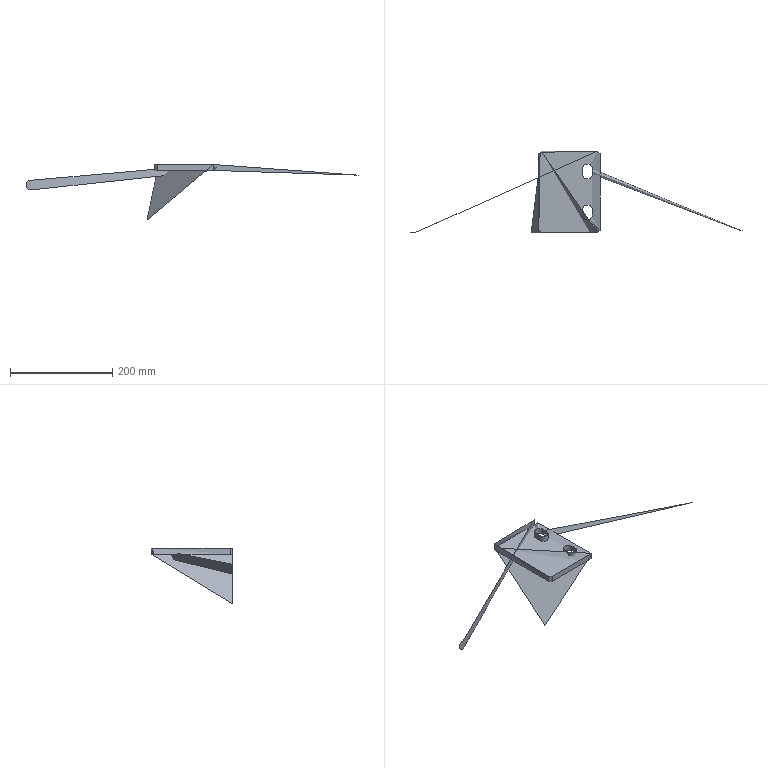Part | STEP file | Stair connecting plate 1 | 1 solid | 18 faces | volume 160302 mm3 | plane 14 | cylinder 4 | commonest cylinder face diameters 19 x4